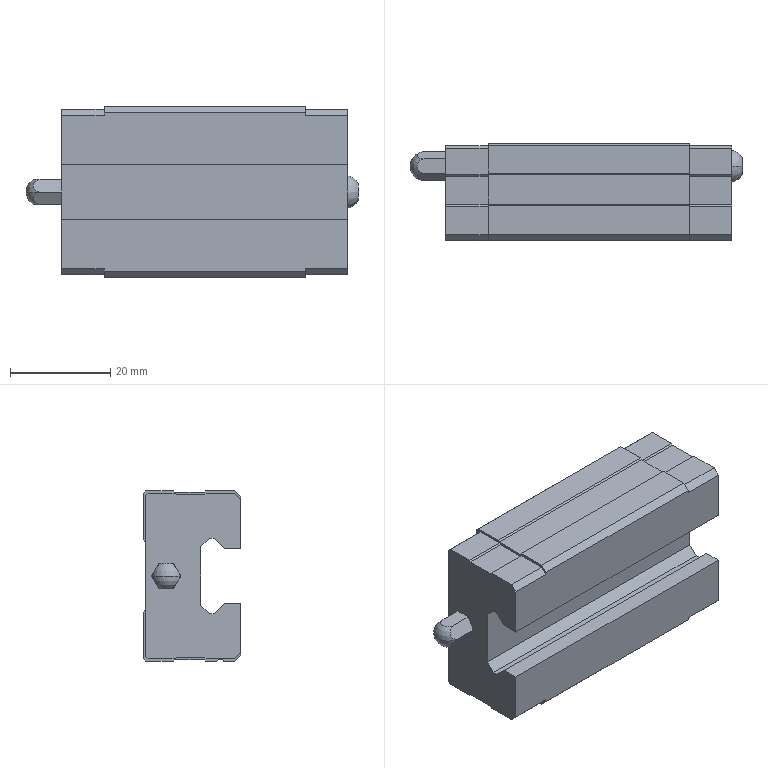Part | STEP file | LSD15BK-HN-N-A-M4 | 1 solid | 109 faces | box 66.3 x 19.5 x 34 mm | volume 30804 mm3 | plane 87 | cylinder 10 | cone 8 | spline 2 | sphere 2 | commonest cylinder face diameters 3.242 x8 1.5 x2